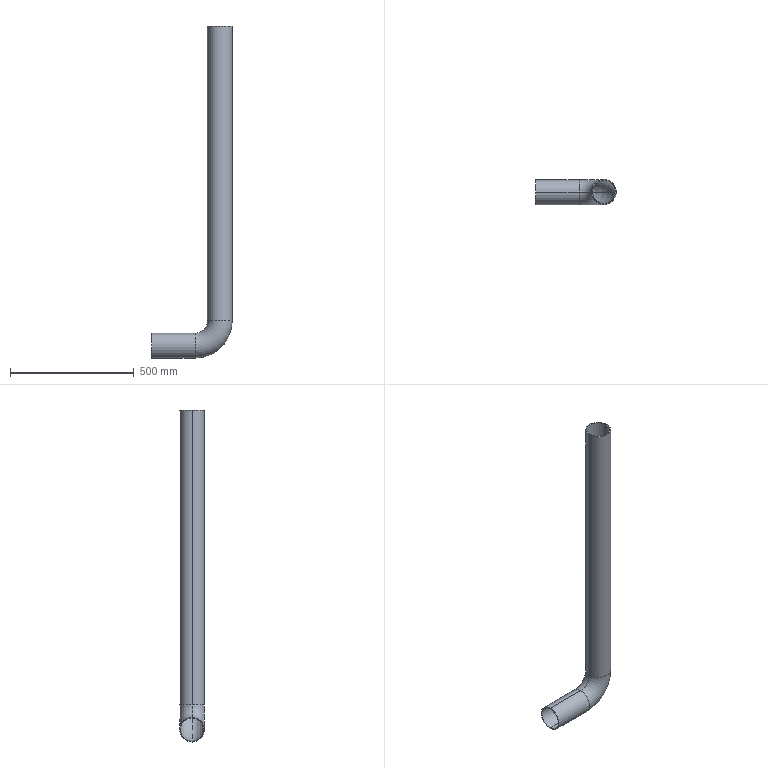Part | SolidWorks | features Shell 1, Sweep 1 | 1 solid | 14 faces | box 325 x 100 x 1340 mm | volume 1391490 mm3 | cylinder 8 | torus 4 | plane 2 | commonest cylinder face diameters 94 x4 100 x4
STEP:
#1=CARTESIAN_POINT('',(-47.,0.,-1190.));
#2=VERTEX_POINT('',#1);
#3=CARTESIAN_POINT('',(47.,0.,-1190.));
#4=VERTEX_POINT('',#3);
#5=CARTESIAN_POINT('',(0.,0.,-1190.));
#6=DIRECTION('',(0.,0.,1.));
#7=DIRECTION('',(-1.,0.,0.));
#8=AXIS2_PLACEMENT_3D('',#5,#6,#7);
#9=CIRCLE('',#8,47.);
#10=EDGE_CURVE('',#2,#4,#9,.T.);
#11=ORIENTED_EDGE('',*,*,#10,.T.);
#12=CARTESIAN_POINT('',(-100.,0.,-1337.));
#13=VERTEX_POINT('',#12);
#14=CARTESIAN_POINT('',(-100.,0.,-1190.));
#15=DIRECTION('',(0.,1.,0.));
#16=DIRECTION('',(0.,0.,1.));
#17=AXIS2_PLACEMENT_3D('',#14,#15,#16);
#18=CIRCLE('',#17,147.);
#19=EDGE_CURVE('',#4,#13,#18,.T.);
#20=ORIENTED_EDGE('',*,*,#19,.T.);
#21=CARTESIAN_POINT('',(-100.,0.,-1243.));
#22=VERTEX_POINT('',#21);
#23=CARTESIAN_POINT('',(-100.,0.,-1290.));
#24=DIRECTION('',(1.,0.,0.));
#25=DIRECTION('',(0.,0.,-1.));
#26=AXIS2_PLACEMENT_3D('',#23,#24,#25);
#27=CIRCLE('',#26,47.);
#28=EDGE_CURVE('',#22,#13,#27,.T.);
#29=ORIENTED_EDGE('',*,*,#28,.F.);
#30=CARTESIAN_POINT('',(-100.,0.,-1190.));
#31=DIRECTION('',(0.,1.,0.));
#32=DIRECTION('',(0.,0.,1.));
#33=AXIS2_PLACEMENT_3D('',#30,#31,#32);
#34=CIRCLE('',#33,53.);
#35=EDGE_CURVE('',#2,#22,#34,.T.);
#36=ORIENTED_EDGE('',*,*,#35,.F.);
#37=EDGE_LOOP('',(#11,#20,#29,#36));
#38=FACE_OUTER_BOUND('',#37,.T.);
#39=CARTESIAN_POINT('',(-100.,0.,-1190.));
#40=DIRECTION('',(0.,1.,0.));
#41=DIRECTION('',(0.,0.,1.));
#42=AXIS2_PLACEMENT_3D('',#39,#40,#41);
#43=TOROIDAL_SURFACE('',#42,100.,47.);
#44=ADVANCED_FACE('',(#38),#43,.F.);
#45=CARTESIAN_POINT('',(50.,0.,-1190.));
#46=VERTEX_POINT('',#45);
#47=CARTESIAN_POINT('',(-50.,0.,-1190.));
#48=VERTEX_POINT('',#47);
#49=CARTESIAN_POINT('',(0.,0.,-1190.));
#50=DIRECTION('',(0.,0.,1.));
#51=DIRECTION('',(1.,0.,0.));
#52=AXIS2_PLACEMENT_3D('',#49,#50,#51);
#53=CIRCLE('',#52,50.);
#54=EDGE_CURVE('',#46,#48,#53,.T.);
#55=ORIENTED_EDGE('',*,*,#54,.F.);
#56=CARTESIAN_POINT('',(-100.,0.,-1340.));
#57=VERTEX_POINT('',#56);
#58=CARTESIAN_POINT('',(-100.,0.,-1190.));
#59=DIRECTION('',(0.,1.,0.));
#60=DIRECTION('',(0.,0.,1.));
#61=AXIS2_PLACEMENT_3D('',#58,#59,#60);
#62=CIRCLE('',#61,150.);
#63=EDGE_CURVE('',#46,#57,#62,.T.);
#64=ORIENTED_EDGE('',*,*,#63,.T.);
#65=CARTESIAN_POINT('',(-100.,0.,-1240.));
#66=VERTEX_POINT('',#65);
#67=CARTESIAN_POINT('',(-100.,0.,-1290.));
#68=DIRECTION('',(1.,0.,0.));
#69=DIRECTION('',(0.,0.,-1.));
#70=AXIS2_PLACEMENT_3D('',#67,#68,#69);
#71=CIRCLE('',#70,50.);
#72=EDGE_CURVE('',#57,#66,#71,.T.);
#73=ORIENTED_EDGE('',*,*,#72,.T.);
#74=CARTESIAN_POINT('',(-100.,0.,-1190.));
#75=DIRECTION('',(0.,1.,0.));
#76=DIRECTION('',(0.,0.,1.));
#77=AXIS2_PLACEMENT_3D('',#74,#75,#76);
#78=CIRCLE('',#77,50.);
#79=EDGE_CURVE('',#48,#66,#78,.T.);
#80=ORIENTED_EDGE('',*,*,#79,.F.);
#81=EDGE_LOOP('',(#55,#64,#73,#80));
#82=FACE_OUTER_BOUND('',#81,.T.);
#83=CARTESIAN_POINT('',(-100.,0.,-1190.));
#84=DIRECTION('',(0.,1.,0.));
#85=DIRECTION('',(0.,0.,1.));
#86=AXIS2_PLACEMENT_3D('',#83,#84,#85);
#87=TOROIDAL_SURFACE('',#86,100.,50.);
#88=ADVANCED_FACE('',(#82),#87,.T.);
#89=ORIENTED_EDGE('',*,*,#28,.T.);
#90=CARTESIAN_POINT('',(-275.,0.,-1337.));
#91=VERTEX_POINT('',#90);
#92=CARTESIAN_POINT('',(-100.,0.,-1337.));
#93=DIRECTION('',(-1.,0.,0.));
#94=VECTOR('',#93,1000.);
#95=LINE('',#92,#94);
#96=EDGE_CURVE('',#13,#91,#95,.T.);
#97=ORIENTED_EDGE('',*,*,#96,.T.);
#98=CARTESIAN_POINT('',(-275.,0.,-1243.));
#99=VERTEX_POINT('',#98);
#100=CARTESIAN_POINT('',(-275.,0.,-1290.));
#101=DIRECTION('',(1.,0.,0.));
#102=DIRECTION('',(0.,0.,-1.));
#103=AXIS2_PLACEMENT_3D('',#100,#101,#102);
#104=CIRCLE('',#103,47.);
#105=EDGE_CURVE('',#99,#91,#104,.T.);
#106=ORIENTED_EDGE('',*,*,#105,.F.);
#107=CARTESIAN_POINT('',(-100.,0.,-1243.));
#108=DIRECTION('',(-1.,0.,0.));
#109=VECTOR('',#108,1000.);
#110=LINE('',#107,#109);
#111=EDGE_CURVE('',#22,#99,#110,.T.);
#112=ORIENTED_EDGE('',*,*,#111,.F.);
#113=EDGE_LOOP('',(#89,#97,#106,#112));
#114=FACE_OUTER_BOUND('',#113,.T.);
#115=CARTESIAN_POINT('',(-100.,0.,-1290.));
#116=DIRECTION('',(-1.,0.,0.));
#117=DIRECTION('',(0.,0.,1.));
#118=AXIS2_PLACEMENT_3D('',#115,#116,#117);
#119=CYLINDRICAL_SURFACE('',#118,47.);
#120=ADVANCED_FACE('',(#114),#119,.F.);
#121=CARTESIAN_POINT('',(-47.,0.,0.));
#122=VERTEX_POINT('',#121);
#123=CARTESIAN_POINT('',(47.,0.,0.));
#124=VERTEX_POINT('',#123);
#125=CARTESIAN_POINT('',(0.,0.,0.));
#126=DIRECTION('',(0.,0.,1.));
#127=DIRECTION('',(1.,0.,0.));
#128=AXIS2_PLACEMENT_3D('',#125,#126,#127);
#129=CIRCLE('',#128,47.);
#130=EDGE_CURVE('',#122,#124,#129,.T.);
#131=ORIENTED_EDGE('',*,*,#130,.T.);
#132=CARTESIAN_POINT('',(47.,0.,0.));
#133=DIRECTION('',(0.,0.,-1.));
#134=VECTOR('',#133,1000.);
#135=LINE('',#132,#134);
#136=EDGE_CURVE('',#124,#4,#135,.T.);
#137=ORIENTED_EDGE('',*,*,#136,.T.);
#138=ORIENTED_EDGE('',*,*,#10,.F.);
#139=CARTESIAN_POINT('',(-47.,0.,0.));
#140=DIRECTION('',(0.,0.,-1.));
#141=VECTOR('',#140,1000.);
#142=LINE('',#139,#141);
#143=EDGE_CURVE('',#122,#2,#142,.T.);
#144=ORIENTED_EDGE('',*,*,#143,.F.);
#145=EDGE_LOOP('',(#131,#137,#138,#144));
#146=FACE_OUTER_BOUND('',#145,.T.);
#147=CARTESIAN_POINT('',(0.,0.,0.));
#148=DIRECTION('',(0.,0.,-1.));
#149=DIRECTION('',(-1.,0.,0.));
#150=AXIS2_PLACEMENT_3D('',#147,#148,#149);
#151=CYLINDRICAL_SURFACE('',#150,47.);
#152=ADVANCED_FACE('',(#146),#151,.F.);
#153=ORIENTED_EDGE('',*,*,#72,.F.);
#154=CARTESIAN_POINT('',(-275.,0.,-1340.));
#155=VERTEX_POINT('',#154);
#156=CARTESIAN_POINT('',(-100.,0.,-1340.));
#157=DIRECTION('',(-1.,0.,0.));
#158=VECTOR('',#157,1000.);
#159=LINE('',#156,#158);
#160=EDGE_CURVE('',#57,#155,#159,.T.);
#161=ORIENTED_EDGE('',*,*,#160,.T.);
#162=CARTESIAN_POINT('',(-275.,0.,-1240.));
#163=VERTEX_POINT('',#162);
#164=CARTESIAN_POINT('',(-275.,0.,-1290.));
#165=DIRECTION('',(1.,0.,0.));
#166=DIRECTION('',(0.,0.,-1.));
#167=AXIS2_PLACEMENT_3D('',#164,#165,#166);
#168=CIRCLE('',#167,50.);
#169=EDGE_CURVE('',#155,#163,#168,.T.);
#170=ORIENTED_EDGE('',*,*,#169,.T.);
#171=CARTESIAN_POINT('',(-100.,0.,-1240.));
#172=DIRECTION('',(-1.,0.,0.));
#173=VECTOR('',#172,1000.);
#174=LINE('',#171,#173);
#175=EDGE_CURVE('',#66,#163,#174,.T.);
#176=ORIENTED_EDGE('',*,*,#175,.F.);
#177=EDGE_LOOP('',(#153,#161,#170,#176));
#178=FACE_OUTER_BOUND('',#177,.T.);
#179=CARTESIAN_POINT('',(-100.,0.,-1290.));
#180=DIRECTION('',(-1.,0.,0.));
#181=DIRECTION('',(0.,0.,1.));
#182=AXIS2_PLACEMENT_3D('',#179,#180,#181);
#183=CYLINDRICAL_SURFACE('',#182,50.);
#184=ADVANCED_FACE('',(#178),#183,.T.);
#185=CARTESIAN_POINT('',(50.,0.,0.));
#186=VERTEX_POINT('',#185);
#187=CARTESIAN_POINT('',(-50.,0.,0.));
#188=VERTEX_POINT('',#187);
#189=CARTESIAN_POINT('',(0.,0.,0.));
#190=DIRECTION('',(0.,0.,1.));
#191=DIRECTION('',(1.,0.,0.));
#192=AXIS2_PLACEMENT_3D('',#189,#190,#191);
#193=CIRCLE('',#192,50.);
#194=EDGE_CURVE('',#186,#188,#193,.T.);
#195=ORIENTED_EDGE('',*,*,#194,.F.);
#196=CARTESIAN_POINT('',(50.,0.,0.));
#197=DIRECTION('',(0.,0.,-1.));
#198=VECTOR('',#197,1000.);
#199=LINE('',#196,#198);
#200=EDGE_CURVE('',#186,#46,#199,.T.);
#201=ORIENTED_EDGE('',*,*,#200,.T.);
#202=ORIENTED_EDGE('',*,*,#54,.T.);
#203=CARTESIAN_POINT('',(-50.,0.,0.));
#204=DIRECTION('',(0.,0.,-1.));
#205=VECTOR('',#204,1000.);
#206=LINE('',#203,#205);
#207=EDGE_CURVE('',#188,#48,#206,.T.);
#208=ORIENTED_EDGE('',*,*,#207,.F.);
#209=EDGE_LOOP('',(#195,#201,#202,#208));
#210=FACE_OUTER_BOUND('',#209,.T.);
#211=CARTESIAN_POINT('',(0.,0.,0.));
#212=DIRECTION('',(0.,0.,-1.));
#213=DIRECTION('',(-1.,0.,0.));
#214=AXIS2_PLACEMENT_3D('',#211,#212,#213);
#215=CYLINDRICAL_SURFACE('',#214,50.);
#216=ADVANCED_FACE('',(#210),#215,.T.);
#217=ORIENTED_EDGE('',*,*,#160,.F.);
#218=CARTESIAN_POINT('',(-100.,0.,-1290.));
#219=DIRECTION('',(1.,0.,0.));
#220=DIRECTION('',(0.,0.,-1.));
#221=AXIS2_PLACEMENT_3D('',#218,#219,#220);
#222=CIRCLE('',#221,50.);
#223=EDGE_CURVE('',#66,#57,#222,.T.);
#224=ORIENTED_EDGE('',*,*,#223,.F.);
#225=ORIENTED_EDGE('',*,*,#175,.T.);
#226=CARTESIAN_POINT('',(-275.,0.,-1290.));
#227=DIRECTION('',(1.,0.,0.));
#228=DIRECTION('',(0.,0.,-1.));
#229=AXIS2_PLACEMENT_3D('',#226,#227,#228);
#230=CIRCLE('',#229,50.);
#231=EDGE_CURVE('',#163,#155,#230,.T.);
#232=ORIENTED_EDGE('',*,*,#231,.T.);
#233=EDGE_LOOP('',(#217,#224,#225,#232));
#234=FACE_OUTER_BOUND('',#233,.T.);
#235=CARTESIAN_POINT('',(-100.,0.,-1290.));
#236=DIRECTION('',(-1.,0.,0.));
#237=DIRECTION('',(0.,0.,1.));
#238=AXIS2_PLACEMENT_3D('',#235,#236,#237);
#239=CYLINDRICAL_SURFACE('',#238,50.);
#240=ADVANCED_FACE('',(#234),#239,.T.);
#241=ORIENTED_EDGE('',*,*,#63,.F.);
#242=CARTESIAN_POINT('',(0.,0.,-1190.));
#243=DIRECTION('',(0.,0.,1.));
#244=DIRECTION('',(1.,0.,0.));
#245=AXIS2_PLACEMENT_3D('',#242,#243,#244);
#246=CIRCLE('',#245,50.);
#247=EDGE_CURVE('',#48,#46,#246,.T.);
#248=ORIENTED_EDGE('',*,*,#247,.F.);
#249=ORIENTED_EDGE('',*,*,#79,.T.);
#250=ORIENTED_EDGE('',*,*,#223,.T.);
#251=EDGE_LOOP('',(#241,#248,#249,#250));
#252=FACE_OUTER_BOUND('',#251,.T.);
#253=CARTESIAN_POINT('',(-100.,0.,-1190.));
#254=DIRECTION('',(0.,1.,0.));
#255=DIRECTION('',(0.,0.,1.));
#256=AXIS2_PLACEMENT_3D('',#253,#254,#255);
#257=TOROIDAL_SURFACE('',#256,100.,50.);
#258=ADVANCED_FACE('',(#252),#257,.T.);
#259=ORIENTED_EDGE('',*,*,#200,.F.);
#260=CARTESIAN_POINT('',(0.,0.,0.));
#261=DIRECTION('',(0.,0.,1.));
#262=DIRECTION('',(1.,0.,0.));
#263=AXIS2_PLACEMENT_3D('',#260,#261,#262);
#264=CIRCLE('',#263,50.);
#265=EDGE_CURVE('',#188,#186,#264,.T.);
#266=ORIENTED_EDGE('',*,*,#265,.F.);
#267=ORIENTED_EDGE('',*,*,#207,.T.);
#268=ORIENTED_EDGE('',*,*,#247,.T.);
#269=EDGE_LOOP('',(#259,#266,#267,#268));
#270=FACE_OUTER_BOUND('',#269,.T.);
#271=CARTESIAN_POINT('',(0.,0.,0.));
#272=DIRECTION('',(0.,0.,-1.));
#273=DIRECTION('',(-1.,0.,0.));
#274=AXIS2_PLACEMENT_3D('',#271,#272,#273);
#275=CYLINDRICAL_SURFACE('',#274,50.);
#276=ADVANCED_FACE('',(#270),#275,.T.);
#277=ORIENTED_EDGE('',*,*,#105,.T.);
#278=CARTESIAN_POINT('',(-275.,0.,-1290.));
#279=DIRECTION('',(1.,0.,0.));
#280=DIRECTION('',(0.,0.,-1.));
#281=AXIS2_PLACEMENT_3D('',#278,#279,#280);
#282=CIRCLE('',#281,47.);
#283=EDGE_CURVE('',#91,#99,#282,.T.);
#284=ORIENTED_EDGE('',*,*,#283,.T.);
#285=EDGE_LOOP('',(#277,#284));
#286=FACE_BOUND('',#285,.T.);
#287=ORIENTED_EDGE('',*,*,#231,.F.);
#288=ORIENTED_EDGE('',*,*,#169,.F.);
#289=EDGE_LOOP('',(#287,#288));
#290=FACE_OUTER_BOUND('',#289,.T.);
#291=CARTESIAN_POINT('',(-275.,0.,-1290.));
#292=DIRECTION('',(1.,0.,0.));
#293=DIRECTION('',(0.,0.,-1.));
#294=AXIS2_PLACEMENT_3D('',#291,#292,#293);
#295=PLANE('',#294);
#296=ADVANCED_FACE('',(#286,#290),#295,.F.);
#297=ORIENTED_EDGE('',*,*,#130,.F.);
#298=CARTESIAN_POINT('',(0.,0.,0.));
#299=DIRECTION('',(0.,0.,1.));
#300=DIRECTION('',(1.,0.,0.));
#301=AXIS2_PLACEMENT_3D('',#298,#299,#300);
#302=CIRCLE('',#301,47.);
#303=EDGE_CURVE('',#124,#122,#302,.T.);
#304=ORIENTED_EDGE('',*,*,#303,.F.);
#305=EDGE_LOOP('',(#297,#304));
#306=FACE_BOUND('',#305,.T.);
#307=ORIENTED_EDGE('',*,*,#265,.T.);
#308=ORIENTED_EDGE('',*,*,#194,.T.);
#309=EDGE_LOOP('',(#307,#308));
#310=FACE_OUTER_BOUND('',#309,.T.);
#311=CARTESIAN_POINT('',(0.,0.,0.));
#312=DIRECTION('',(0.,0.,1.));
#313=DIRECTION('',(1.,0.,0.));
#314=AXIS2_PLACEMENT_3D('',#311,#312,#313);
#315=PLANE('',#314);
#316=ADVANCED_FACE('',(#306,#310),#315,.T.);
#317=ORIENTED_EDGE('',*,*,#96,.F.);
#318=CARTESIAN_POINT('',(-100.,0.,-1290.));
#319=DIRECTION('',(1.,0.,0.));
#320=DIRECTION('',(0.,0.,-1.));
#321=AXIS2_PLACEMENT_3D('',#318,#319,#320);
#322=CIRCLE('',#321,47.);
#323=EDGE_CURVE('',#13,#22,#322,.T.);
#324=ORIENTED_EDGE('',*,*,#323,.T.);
#325=ORIENTED_EDGE('',*,*,#111,.T.);
#326=ORIENTED_EDGE('',*,*,#283,.F.);
#327=EDGE_LOOP('',(#317,#324,#325,#326));
#328=FACE_OUTER_BOUND('',#327,.T.);
#329=CARTESIAN_POINT('',(-100.,0.,-1290.));
#330=DIRECTION('',(-1.,0.,0.));
#331=DIRECTION('',(0.,0.,1.));
#332=AXIS2_PLACEMENT_3D('',#329,#330,#331);
#333=CYLINDRICAL_SURFACE('',#332,47.);
#334=ADVANCED_FACE('',(#328),#333,.F.);
#335=ORIENTED_EDGE('',*,*,#19,.F.);
#336=CARTESIAN_POINT('',(0.,0.,-1190.));
#337=DIRECTION('',(0.,0.,1.));
#338=DIRECTION('',(-1.,0.,0.));
#339=AXIS2_PLACEMENT_3D('',#336,#337,#338);
#340=CIRCLE('',#339,47.);
#341=EDGE_CURVE('',#4,#2,#340,.T.);
#342=ORIENTED_EDGE('',*,*,#341,.T.);
#343=ORIENTED_EDGE('',*,*,#35,.T.);
#344=ORIENTED_EDGE('',*,*,#323,.F.);
#345=EDGE_LOOP('',(#335,#342,#343,#344));
#346=FACE_OUTER_BOUND('',#345,.T.);
#347=CARTESIAN_POINT('',(-100.,0.,-1190.));
#348=DIRECTION('',(0.,1.,0.));
#349=DIRECTION('',(0.,0.,1.));
#350=AXIS2_PLACEMENT_3D('',#347,#348,#349);
#351=TOROIDAL_SURFACE('',#350,100.,47.);
#352=ADVANCED_FACE('',(#346),#351,.F.);
#353=ORIENTED_EDGE('',*,*,#136,.F.);
#354=ORIENTED_EDGE('',*,*,#303,.T.);
#355=ORIENTED_EDGE('',*,*,#143,.T.);
#356=ORIENTED_EDGE('',*,*,#341,.F.);
#357=EDGE_LOOP('',(#353,#354,#355,#356));
#358=FACE_OUTER_BOUND('',#357,.T.);
#359=CARTESIAN_POINT('',(0.,0.,0.));
#360=DIRECTION('',(0.,0.,-1.));
#361=DIRECTION('',(-1.,0.,0.));
#362=AXIS2_PLACEMENT_3D('',#359,#360,#361);
#363=CYLINDRICAL_SURFACE('',#362,47.);
#364=ADVANCED_FACE('',(#358),#363,.F.);
#365=CLOSED_SHELL('',(#44,#88,#120,#152,#184,#216,#240,#258,#276,#296,#316,#334,#352,#364));
#366=MANIFOLD_SOLID_BREP('',#365);
#367=CARTESIAN_POINT('',(0.,0.,0.));
#368=DIRECTION('',(0.,0.,1.));
#369=DIRECTION('',(1.,0.,0.));
#370=AXIS2_PLACEMENT_3D('',#367,#368,#369);
#371=(LENGTH_UNIT()NAMED_UNIT(*)SI_UNIT(.MILLI.,.METRE.));
#372=UNCERTAINTY_MEASURE_WITH_UNIT(LENGTH_MEASURE(0.00001),#371,'','');
#373=(NAMED_UNIT(*)PLANE_ANGLE_UNIT()SI_UNIT($,.RADIAN.));
#374=(NAMED_UNIT(*)SI_UNIT($,.STERADIAN.)SOLID_ANGLE_UNIT());
#375=(GEOMETRIC_REPRESENTATION_CONTEXT(3)GLOBAL_UNCERTAINTY_ASSIGNED_CONTEXT((#372))GLOBAL_UNIT_ASSIGNED_CONTEXT((#371,#373,#374))REPRESENTATION_CONTEXT('',''));
#376=ADVANCED_BREP_SHAPE_REPRESENTATION('',(#366,#370),#375);